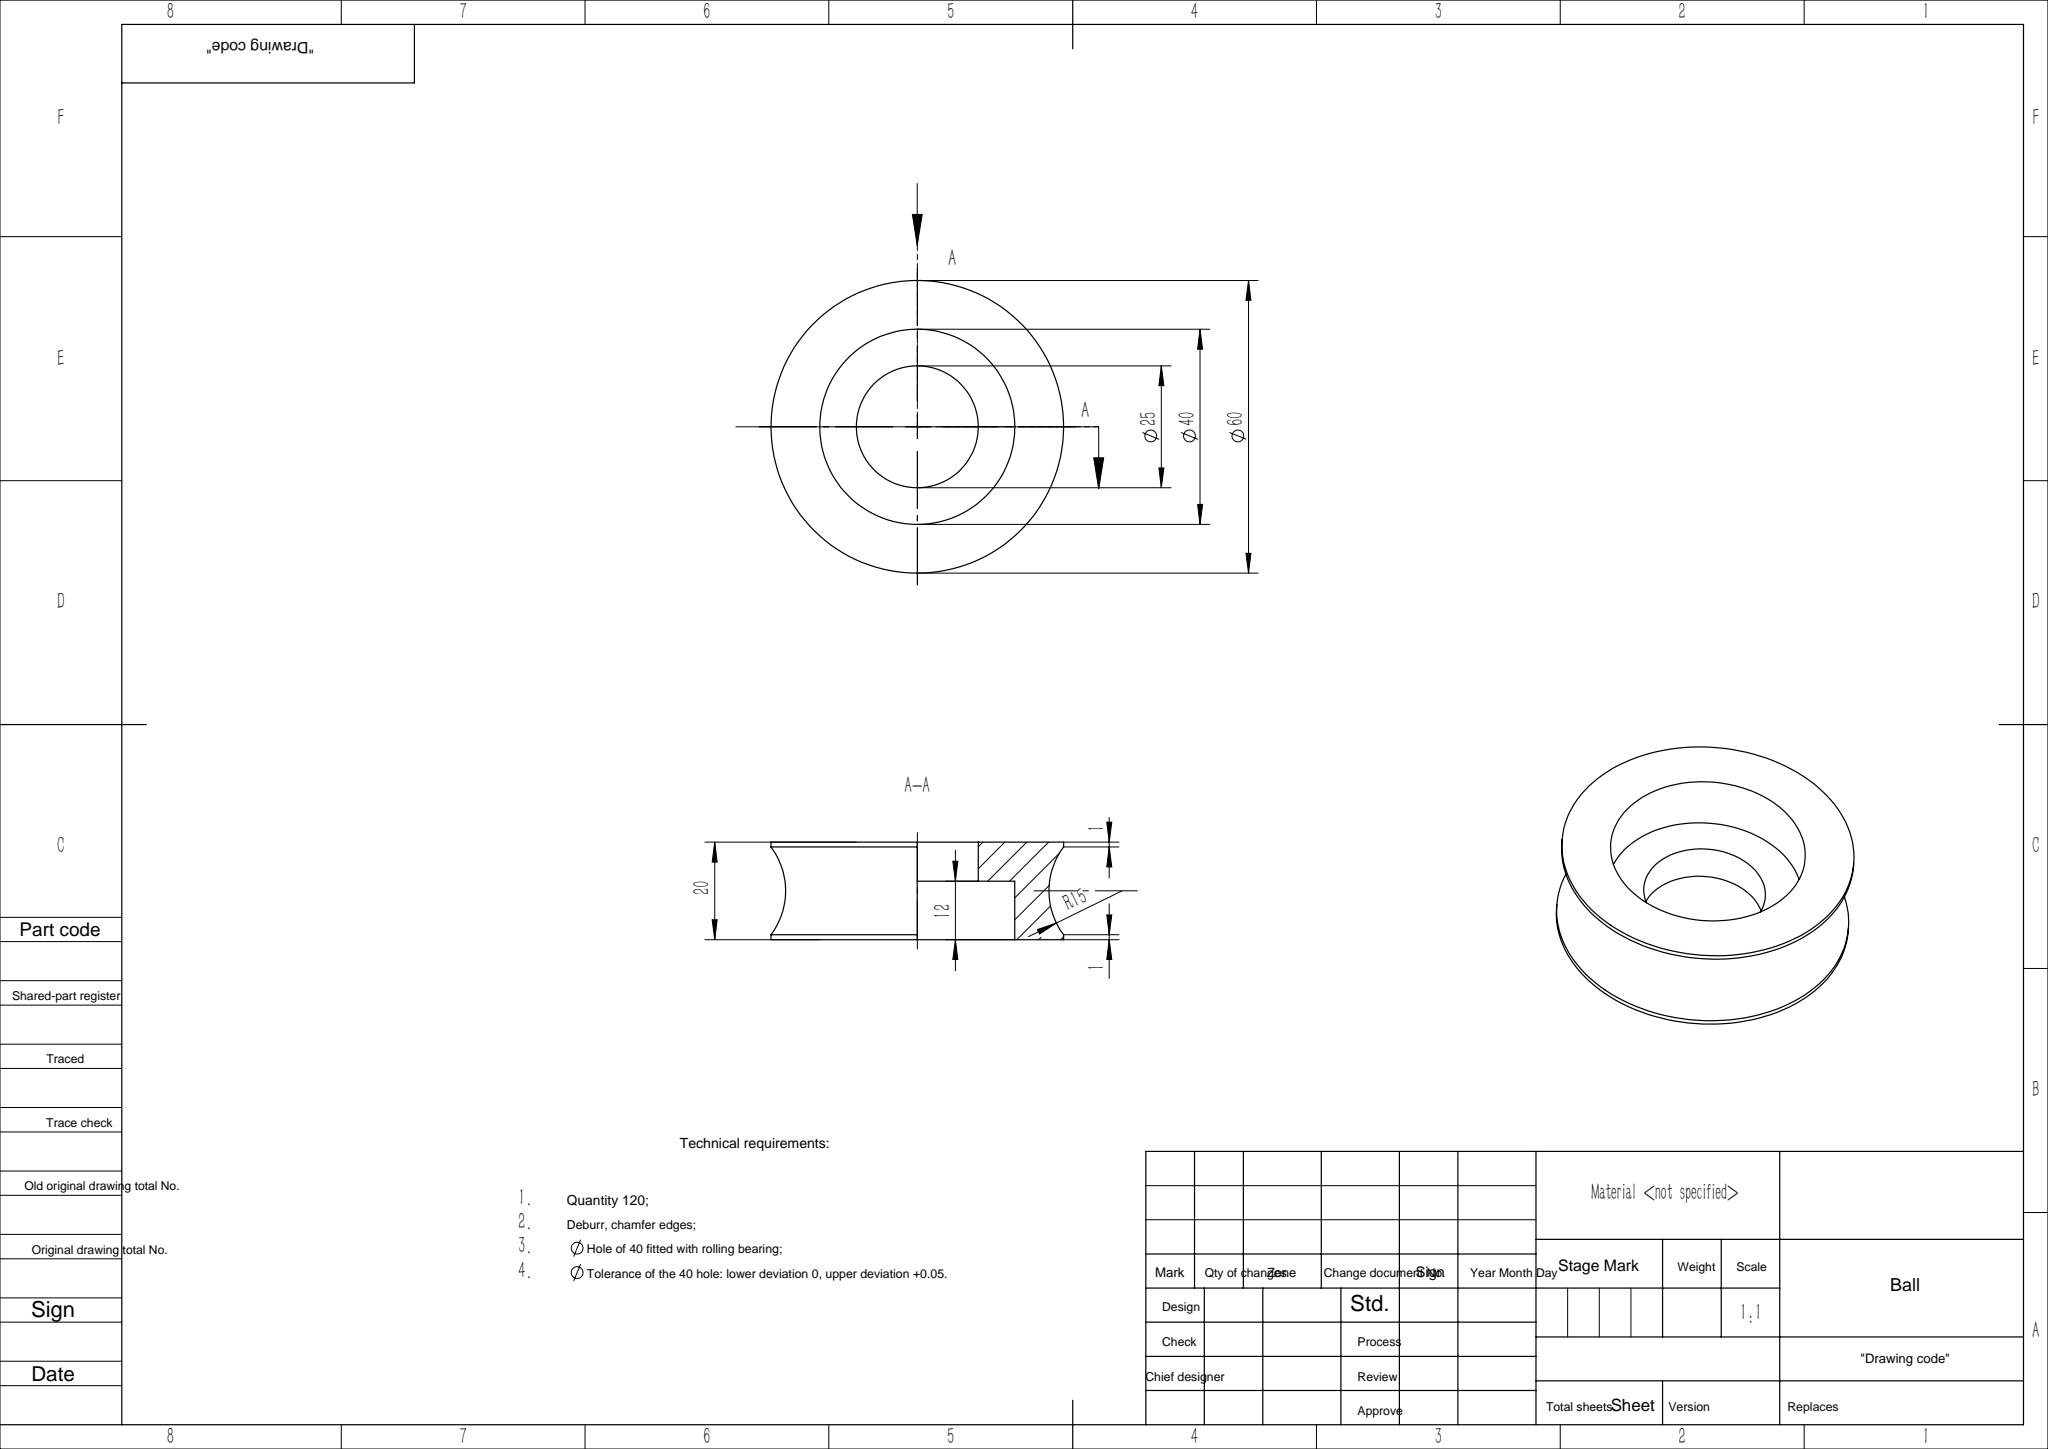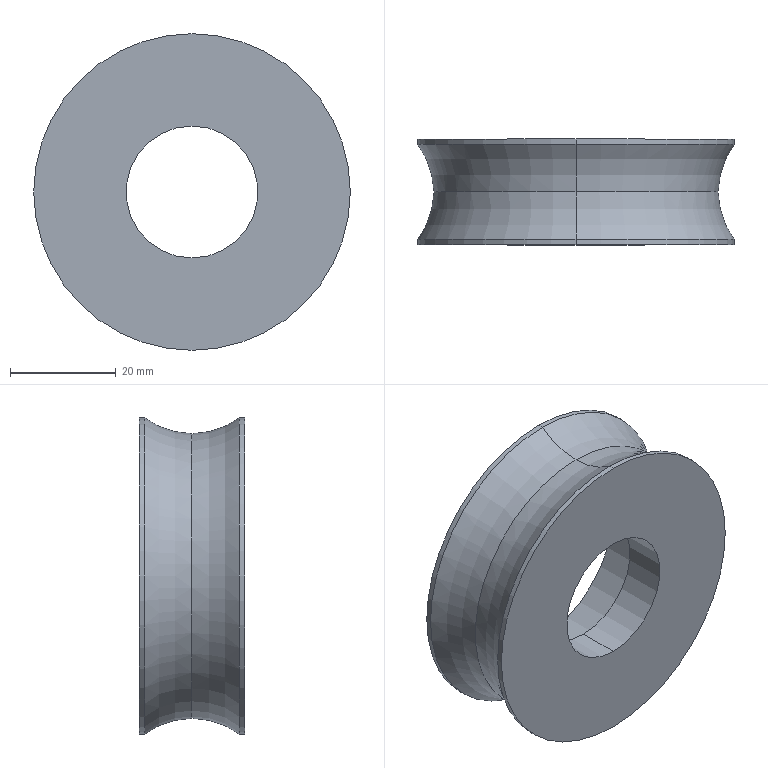Part | SolidWorks | features ICE 2, Extrusion 1, RevCut 1 | 1 solid | 15 faces | box 60 x 20 x 60 mm | volume 30888 mm3 | cylinder 8 | torus 4 | plane 3 | commonest cylinder face diameters 60 x4 25 x2 40 x2
STEP:
#1=CARTESIAN_POINT('',(0.,1.,-30.));
#2=VERTEX_POINT('',#1);
#3=CARTESIAN_POINT('',(0.,10.,-27.));
#4=VERTEX_POINT('',#3);
#5=CARTESIAN_POINT('',(0.,10.,-42.));
#6=DIRECTION('',(-1.,0.,0.));
#7=DIRECTION('',(0.,0.,1.));
#8=AXIS2_PLACEMENT_3D('',#5,#6,#7);
#9=CIRCLE('',#8,15.);
#10=EDGE_CURVE('',#2,#4,#9,.T.);
#11=ORIENTED_EDGE('',*,*,#10,.T.);
#12=CARTESIAN_POINT('',(0.,10.,27.));
#13=VERTEX_POINT('',#12);
#14=CARTESIAN_POINT('',(0.,10.,0.));
#15=DIRECTION('',(0.,-1.,0.));
#16=DIRECTION('',(0.,0.,-1.));
#17=AXIS2_PLACEMENT_3D('',#14,#15,#16);
#18=CIRCLE('',#17,27.);
#19=EDGE_CURVE('',#4,#13,#18,.T.);
#20=ORIENTED_EDGE('',*,*,#19,.T.);
#21=CARTESIAN_POINT('',(0.,1.,30.));
#22=VERTEX_POINT('',#21);
#23=CARTESIAN_POINT('',(0.,10.,42.));
#24=DIRECTION('',(1.,0.,0.));
#25=DIRECTION('',(0.,0.,-1.));
#26=AXIS2_PLACEMENT_3D('',#23,#24,#25);
#27=CIRCLE('',#26,15.);
#28=EDGE_CURVE('',#22,#13,#27,.T.);
#29=ORIENTED_EDGE('',*,*,#28,.F.);
#30=CARTESIAN_POINT('',(0.,1.,0.));
#31=DIRECTION('',(0.,-1.,0.));
#32=DIRECTION('',(0.,0.,1.));
#33=AXIS2_PLACEMENT_3D('',#30,#31,#32);
#34=CIRCLE('',#33,30.);
#35=EDGE_CURVE('',#2,#22,#34,.T.);
#36=ORIENTED_EDGE('',*,*,#35,.F.);
#37=EDGE_LOOP('',(#11,#20,#29,#36));
#38=FACE_OUTER_BOUND('',#37,.T.);
#39=CARTESIAN_POINT('',(0.,10.,0.));
#40=DIRECTION('',(0.,-1.,0.));
#41=DIRECTION('',(0.,0.,-1.));
#42=AXIS2_PLACEMENT_3D('',#39,#40,#41);
#43=TOROIDAL_SURFACE('',#42,42.,15.);
#44=ADVANCED_FACE('',(#38),#43,.F.);
#45=ORIENTED_EDGE('',*,*,#28,.T.);
#46=CARTESIAN_POINT('',(0.,10.,0.));
#47=DIRECTION('',(0.,-1.,0.));
#48=DIRECTION('',(0.,0.,-1.));
#49=AXIS2_PLACEMENT_3D('',#46,#47,#48);
#50=CIRCLE('',#49,27.);
#51=EDGE_CURVE('',#13,#4,#50,.T.);
#52=ORIENTED_EDGE('',*,*,#51,.T.);
#53=ORIENTED_EDGE('',*,*,#10,.F.);
#54=CARTESIAN_POINT('',(0.,1.,0.));
#55=DIRECTION('',(0.,-1.,0.));
#56=DIRECTION('',(0.,0.,1.));
#57=AXIS2_PLACEMENT_3D('',#54,#55,#56);
#58=CIRCLE('',#57,30.);
#59=EDGE_CURVE('',#22,#2,#58,.T.);
#60=ORIENTED_EDGE('',*,*,#59,.F.);
#61=EDGE_LOOP('',(#45,#52,#53,#60));
#62=FACE_OUTER_BOUND('',#61,.T.);
#63=CARTESIAN_POINT('',(0.,10.,0.));
#64=DIRECTION('',(0.,-1.,0.));
#65=DIRECTION('',(0.,0.,-1.));
#66=AXIS2_PLACEMENT_3D('',#63,#64,#65);
#67=TOROIDAL_SURFACE('',#66,42.,15.);
#68=ADVANCED_FACE('',(#62),#67,.F.);
#69=ORIENTED_EDGE('',*,*,#51,.F.);
#70=CARTESIAN_POINT('',(0.,19.,30.));
#71=VERTEX_POINT('',#70);
#72=CARTESIAN_POINT('',(0.,10.,42.));
#73=DIRECTION('',(1.,0.,0.));
#74=DIRECTION('',(0.,0.,-1.));
#75=AXIS2_PLACEMENT_3D('',#72,#73,#74);
#76=CIRCLE('',#75,15.);
#77=EDGE_CURVE('',#13,#71,#76,.T.);
#78=ORIENTED_EDGE('',*,*,#77,.T.);
#79=CARTESIAN_POINT('',(0.,19.,-30.));
#80=VERTEX_POINT('',#79);
#81=CARTESIAN_POINT('',(0.,19.,0.));
#82=DIRECTION('',(0.,1.,0.));
#83=DIRECTION('',(0.,0.,-1.));
#84=AXIS2_PLACEMENT_3D('',#81,#82,#83);
#85=CIRCLE('',#84,30.);
#86=EDGE_CURVE('',#80,#71,#85,.T.);
#87=ORIENTED_EDGE('',*,*,#86,.F.);
#88=CARTESIAN_POINT('',(0.,10.,-42.));
#89=DIRECTION('',(-1.,0.,0.));
#90=DIRECTION('',(0.,0.,1.));
#91=AXIS2_PLACEMENT_3D('',#88,#89,#90);
#92=CIRCLE('',#91,15.);
#93=EDGE_CURVE('',#4,#80,#92,.T.);
#94=ORIENTED_EDGE('',*,*,#93,.F.);
#95=EDGE_LOOP('',(#69,#78,#87,#94));
#96=FACE_OUTER_BOUND('',#95,.T.);
#97=CARTESIAN_POINT('',(0.,10.,0.));
#98=DIRECTION('',(0.,-1.,0.));
#99=DIRECTION('',(0.,0.,-1.));
#100=AXIS2_PLACEMENT_3D('',#97,#98,#99);
#101=TOROIDAL_SURFACE('',#100,42.,15.);
#102=ADVANCED_FACE('',(#96),#101,.F.);
#103=CARTESIAN_POINT('',(0.,0.,-12.5));
#104=VERTEX_POINT('',#103);
#105=CARTESIAN_POINT('',(0.,0.,12.5));
#106=VERTEX_POINT('',#105);
#107=CARTESIAN_POINT('',(0.,0.,0.));
#108=DIRECTION('',(0.,1.,0.));
#109=DIRECTION('',(0.,0.,1.));
#110=AXIS2_PLACEMENT_3D('',#107,#108,#109);
#111=CIRCLE('',#110,12.5);
#112=EDGE_CURVE('',#104,#106,#111,.T.);
#113=ORIENTED_EDGE('',*,*,#112,.F.);
#114=CARTESIAN_POINT('',(0.,8.,-12.5));
#115=VERTEX_POINT('',#114);
#116=CARTESIAN_POINT('',(0.,0.,-12.5));
#117=DIRECTION('',(0.,1.,0.));
#118=VECTOR('',#117,1000.);
#119=LINE('',#116,#118);
#120=EDGE_CURVE('',#104,#115,#119,.T.);
#121=ORIENTED_EDGE('',*,*,#120,.T.);
#122=CARTESIAN_POINT('',(0.,8.,12.5));
#123=VERTEX_POINT('',#122);
#124=CARTESIAN_POINT('',(0.,8.,0.));
#125=DIRECTION('',(0.,1.,0.));
#126=DIRECTION('',(0.,0.,1.));
#127=AXIS2_PLACEMENT_3D('',#124,#125,#126);
#128=CIRCLE('',#127,12.5);
#129=EDGE_CURVE('',#115,#123,#128,.T.);
#130=ORIENTED_EDGE('',*,*,#129,.T.);
#131=CARTESIAN_POINT('',(0.,0.,12.5));
#132=DIRECTION('',(0.,1.,0.));
#133=VECTOR('',#132,1000.);
#134=LINE('',#131,#133);
#135=EDGE_CURVE('',#106,#123,#134,.T.);
#136=ORIENTED_EDGE('',*,*,#135,.F.);
#137=EDGE_LOOP('',(#113,#121,#130,#136));
#138=FACE_OUTER_BOUND('',#137,.T.);
#139=CARTESIAN_POINT('',(0.,0.,0.));
#140=DIRECTION('',(0.,1.,0.));
#141=DIRECTION('',(0.,0.,1.));
#142=AXIS2_PLACEMENT_3D('',#139,#140,#141);
#143=CYLINDRICAL_SURFACE('',#142,12.5);
#144=ADVANCED_FACE('',(#138),#143,.F.);
#145=CARTESIAN_POINT('',(0.,8.,-20.));
#146=VERTEX_POINT('',#145);
#147=CARTESIAN_POINT('',(0.,8.,20.));
#148=VERTEX_POINT('',#147);
#149=CARTESIAN_POINT('',(0.,8.,0.));
#150=DIRECTION('',(0.,1.,0.));
#151=DIRECTION('',(0.,0.,1.));
#152=AXIS2_PLACEMENT_3D('',#149,#150,#151);
#153=CIRCLE('',#152,20.);
#154=EDGE_CURVE('',#146,#148,#153,.T.);
#155=ORIENTED_EDGE('',*,*,#154,.F.);
#156=CARTESIAN_POINT('',(0.,20.,-20.));
#157=VERTEX_POINT('',#156);
#158=CARTESIAN_POINT('',(0.,8.,-20.));
#159=DIRECTION('',(0.,1.,0.));
#160=VECTOR('',#159,1000.);
#161=LINE('',#158,#160);
#162=EDGE_CURVE('',#146,#157,#161,.T.);
#163=ORIENTED_EDGE('',*,*,#162,.T.);
#164=CARTESIAN_POINT('',(0.,20.,20.));
#165=VERTEX_POINT('',#164);
#166=CARTESIAN_POINT('',(0.,20.,0.));
#167=DIRECTION('',(0.,1.,0.));
#168=DIRECTION('',(0.,0.,1.));
#169=AXIS2_PLACEMENT_3D('',#166,#167,#168);
#170=CIRCLE('',#169,20.);
#171=EDGE_CURVE('',#157,#165,#170,.T.);
#172=ORIENTED_EDGE('',*,*,#171,.T.);
#173=CARTESIAN_POINT('',(0.,8.,20.));
#174=DIRECTION('',(0.,1.,0.));
#175=VECTOR('',#174,1000.);
#176=LINE('',#173,#175);
#177=EDGE_CURVE('',#148,#165,#176,.T.);
#178=ORIENTED_EDGE('',*,*,#177,.F.);
#179=EDGE_LOOP('',(#155,#163,#172,#178));
#180=FACE_OUTER_BOUND('',#179,.T.);
#181=CARTESIAN_POINT('',(0.,8.,0.));
#182=DIRECTION('',(0.,1.,0.));
#183=DIRECTION('',(0.,0.,1.));
#184=AXIS2_PLACEMENT_3D('',#181,#182,#183);
#185=CYLINDRICAL_SURFACE('',#184,20.);
#186=ADVANCED_FACE('',(#180),#185,.F.);
#187=CARTESIAN_POINT('',(0.,20.,30.));
#188=VERTEX_POINT('',#187);
#189=CARTESIAN_POINT('',(0.,20.,-30.));
#190=VERTEX_POINT('',#189);
#191=CARTESIAN_POINT('',(0.,20.,0.));
#192=DIRECTION('',(0.,1.,0.));
#193=DIRECTION('',(0.,0.,1.));
#194=AXIS2_PLACEMENT_3D('',#191,#192,#193);
#195=CIRCLE('',#194,30.);
#196=EDGE_CURVE('',#188,#190,#195,.T.);
#197=ORIENTED_EDGE('',*,*,#196,.F.);
#198=CARTESIAN_POINT('',(0.,20.,30.));
#199=DIRECTION('',(0.,-1.,0.));
#200=VECTOR('',#199,1000.);
#201=LINE('',#198,#200);
#202=EDGE_CURVE('',#188,#71,#201,.T.);
#203=ORIENTED_EDGE('',*,*,#202,.T.);
#204=CARTESIAN_POINT('',(0.,19.,0.));
#205=DIRECTION('',(0.,1.,0.));
#206=DIRECTION('',(0.,0.,-1.));
#207=AXIS2_PLACEMENT_3D('',#204,#205,#206);
#208=CIRCLE('',#207,30.);
#209=EDGE_CURVE('',#71,#80,#208,.T.);
#210=ORIENTED_EDGE('',*,*,#209,.T.);
#211=CARTESIAN_POINT('',(0.,20.,-30.));
#212=DIRECTION('',(0.,-1.,0.));
#213=VECTOR('',#212,1000.);
#214=LINE('',#211,#213);
#215=EDGE_CURVE('',#190,#80,#214,.T.);
#216=ORIENTED_EDGE('',*,*,#215,.F.);
#217=EDGE_LOOP('',(#197,#203,#210,#216));
#218=FACE_OUTER_BOUND('',#217,.T.);
#219=CARTESIAN_POINT('',(0.,20.,0.));
#220=DIRECTION('',(0.,-1.,0.));
#221=DIRECTION('',(0.,0.,-1.));
#222=AXIS2_PLACEMENT_3D('',#219,#220,#221);
#223=CYLINDRICAL_SURFACE('',#222,30.);
#224=ADVANCED_FACE('',(#218),#223,.T.);
#225=ORIENTED_EDGE('',*,*,#35,.T.);
#226=CARTESIAN_POINT('',(0.,0.,30.));
#227=VERTEX_POINT('',#226);
#228=CARTESIAN_POINT('',(0.,20.,30.));
#229=DIRECTION('',(0.,-1.,0.));
#230=VECTOR('',#229,1000.);
#231=LINE('',#228,#230);
#232=EDGE_CURVE('',#22,#227,#231,.T.);
#233=ORIENTED_EDGE('',*,*,#232,.T.);
#234=CARTESIAN_POINT('',(0.,0.,-30.));
#235=VERTEX_POINT('',#234);
#236=CARTESIAN_POINT('',(0.,0.,0.));
#237=DIRECTION('',(0.,1.,0.));
#238=DIRECTION('',(0.,0.,1.));
#239=AXIS2_PLACEMENT_3D('',#236,#237,#238);
#240=CIRCLE('',#239,30.);
#241=EDGE_CURVE('',#227,#235,#240,.T.);
#242=ORIENTED_EDGE('',*,*,#241,.T.);
#243=CARTESIAN_POINT('',(0.,20.,-30.));
#244=DIRECTION('',(0.,-1.,0.));
#245=VECTOR('',#244,1000.);
#246=LINE('',#243,#245);
#247=EDGE_CURVE('',#2,#235,#246,.T.);
#248=ORIENTED_EDGE('',*,*,#247,.F.);
#249=EDGE_LOOP('',(#225,#233,#242,#248));
#250=FACE_OUTER_BOUND('',#249,.T.);
#251=CARTESIAN_POINT('',(0.,20.,0.));
#252=DIRECTION('',(0.,-1.,0.));
#253=DIRECTION('',(0.,0.,-1.));
#254=AXIS2_PLACEMENT_3D('',#251,#252,#253);
#255=CYLINDRICAL_SURFACE('',#254,30.);
#256=ADVANCED_FACE('',(#250),#255,.T.);
#257=ORIENTED_EDGE('',*,*,#232,.F.);
#258=ORIENTED_EDGE('',*,*,#59,.T.);
#259=ORIENTED_EDGE('',*,*,#247,.T.);
#260=CARTESIAN_POINT('',(0.,0.,0.));
#261=DIRECTION('',(0.,1.,0.));
#262=DIRECTION('',(0.,0.,1.));
#263=AXIS2_PLACEMENT_3D('',#260,#261,#262);
#264=CIRCLE('',#263,30.);
#265=EDGE_CURVE('',#235,#227,#264,.T.);
#266=ORIENTED_EDGE('',*,*,#265,.T.);
#267=EDGE_LOOP('',(#257,#258,#259,#266));
#268=FACE_OUTER_BOUND('',#267,.T.);
#269=CARTESIAN_POINT('',(0.,20.,0.));
#270=DIRECTION('',(0.,-1.,0.));
#271=DIRECTION('',(0.,0.,-1.));
#272=AXIS2_PLACEMENT_3D('',#269,#270,#271);
#273=CYLINDRICAL_SURFACE('',#272,30.);
#274=ADVANCED_FACE('',(#268),#273,.T.);
#275=ORIENTED_EDGE('',*,*,#202,.F.);
#276=CARTESIAN_POINT('',(0.,20.,0.));
#277=DIRECTION('',(0.,1.,0.));
#278=DIRECTION('',(0.,0.,1.));
#279=AXIS2_PLACEMENT_3D('',#276,#277,#278);
#280=CIRCLE('',#279,30.);
#281=EDGE_CURVE('',#190,#188,#280,.T.);
#282=ORIENTED_EDGE('',*,*,#281,.F.);
#283=ORIENTED_EDGE('',*,*,#215,.T.);
#284=ORIENTED_EDGE('',*,*,#86,.T.);
#285=EDGE_LOOP('',(#275,#282,#283,#284));
#286=FACE_OUTER_BOUND('',#285,.T.);
#287=CARTESIAN_POINT('',(0.,20.,0.));
#288=DIRECTION('',(0.,-1.,0.));
#289=DIRECTION('',(0.,0.,-1.));
#290=AXIS2_PLACEMENT_3D('',#287,#288,#289);
#291=CYLINDRICAL_SURFACE('',#290,30.);
#292=ADVANCED_FACE('',(#286),#291,.T.);
#293=CARTESIAN_POINT('',(0.,20.,0.));
#294=DIRECTION('',(0.,1.,0.));
#295=DIRECTION('',(0.,0.,1.));
#296=AXIS2_PLACEMENT_3D('',#293,#294,#295);
#297=CIRCLE('',#296,20.);
#298=EDGE_CURVE('',#165,#157,#297,.T.);
#299=ORIENTED_EDGE('',*,*,#298,.F.);
#300=ORIENTED_EDGE('',*,*,#171,.F.);
#301=EDGE_LOOP('',(#299,#300));
#302=FACE_BOUND('',#301,.T.);
#303=ORIENTED_EDGE('',*,*,#281,.T.);
#304=ORIENTED_EDGE('',*,*,#196,.T.);
#305=EDGE_LOOP('',(#303,#304));
#306=FACE_OUTER_BOUND('',#305,.T.);
#307=CARTESIAN_POINT('',(0.,20.,0.));
#308=DIRECTION('',(0.,1.,0.));
#309=DIRECTION('',(0.,0.,1.));
#310=AXIS2_PLACEMENT_3D('',#307,#308,#309);
#311=PLANE('',#310);
#312=ADVANCED_FACE('',(#302,#306),#311,.T.);
#313=CARTESIAN_POINT('',(0.,0.,0.));
#314=DIRECTION('',(0.,1.,0.));
#315=DIRECTION('',(0.,0.,1.));
#316=AXIS2_PLACEMENT_3D('',#313,#314,#315);
#317=CIRCLE('',#316,12.5);
#318=EDGE_CURVE('',#106,#104,#317,.T.);
#319=ORIENTED_EDGE('',*,*,#318,.T.);
#320=ORIENTED_EDGE('',*,*,#112,.T.);
#321=EDGE_LOOP('',(#319,#320));
#322=FACE_BOUND('',#321,.T.);
#323=ORIENTED_EDGE('',*,*,#265,.F.);
#324=ORIENTED_EDGE('',*,*,#241,.F.);
#325=EDGE_LOOP('',(#323,#324));
#326=FACE_OUTER_BOUND('',#325,.T.);
#327=CARTESIAN_POINT('',(0.,0.,0.));
#328=DIRECTION('',(0.,1.,0.));
#329=DIRECTION('',(0.,0.,1.));
#330=AXIS2_PLACEMENT_3D('',#327,#328,#329);
#331=PLANE('',#330);
#332=ADVANCED_FACE('',(#322,#326),#331,.F.);
#333=ORIENTED_EDGE('',*,*,#162,.F.);
#334=CARTESIAN_POINT('',(0.,8.,0.));
#335=DIRECTION('',(0.,1.,0.));
#336=DIRECTION('',(0.,0.,1.));
#337=AXIS2_PLACEMENT_3D('',#334,#335,#336);
#338=CIRCLE('',#337,20.);
#339=EDGE_CURVE('',#148,#146,#338,.T.);
#340=ORIENTED_EDGE('',*,*,#339,.F.);
#341=ORIENTED_EDGE('',*,*,#177,.T.);
#342=ORIENTED_EDGE('',*,*,#298,.T.);
#343=EDGE_LOOP('',(#333,#340,#341,#342));
#344=FACE_OUTER_BOUND('',#343,.T.);
#345=CARTESIAN_POINT('',(0.,8.,0.));
#346=DIRECTION('',(0.,1.,0.));
#347=DIRECTION('',(0.,0.,1.));
#348=AXIS2_PLACEMENT_3D('',#345,#346,#347);
#349=CYLINDRICAL_SURFACE('',#348,20.);
#350=ADVANCED_FACE('',(#344),#349,.F.);
#351=CARTESIAN_POINT('',(0.,8.,0.));
#352=DIRECTION('',(0.,1.,0.));
#353=DIRECTION('',(0.,0.,1.));
#354=AXIS2_PLACEMENT_3D('',#351,#352,#353);
#355=CIRCLE('',#354,12.5);
#356=EDGE_CURVE('',#123,#115,#355,.T.);
#357=ORIENTED_EDGE('',*,*,#356,.F.);
#358=ORIENTED_EDGE('',*,*,#129,.F.);
#359=EDGE_LOOP('',(#357,#358));
#360=FACE_BOUND('',#359,.T.);
#361=ORIENTED_EDGE('',*,*,#339,.T.);
#362=ORIENTED_EDGE('',*,*,#154,.T.);
#363=EDGE_LOOP('',(#361,#362));
#364=FACE_OUTER_BOUND('',#363,.T.);
#365=CARTESIAN_POINT('',(0.,8.,0.));
#366=DIRECTION('',(0.,1.,0.));
#367=DIRECTION('',(0.,0.,1.));
#368=AXIS2_PLACEMENT_3D('',#365,#366,#367);
#369=PLANE('',#368);
#370=ADVANCED_FACE('',(#360,#364),#369,.T.);
#371=ORIENTED_EDGE('',*,*,#120,.F.);
#372=ORIENTED_EDGE('',*,*,#318,.F.);
#373=ORIENTED_EDGE('',*,*,#135,.T.);
#374=ORIENTED_EDGE('',*,*,#356,.T.);
#375=EDGE_LOOP('',(#371,#372,#373,#374));
#376=FACE_OUTER_BOUND('',#375,.T.);
#377=CARTESIAN_POINT('',(0.,0.,0.));
#378=DIRECTION('',(0.,1.,0.));
#379=DIRECTION('',(0.,0.,1.));
#380=AXIS2_PLACEMENT_3D('',#377,#378,#379);
#381=CYLINDRICAL_SURFACE('',#380,12.5);
#382=ADVANCED_FACE('',(#376),#381,.F.);
#383=ORIENTED_EDGE('',*,*,#19,.F.);
#384=ORIENTED_EDGE('',*,*,#93,.T.);
#385=ORIENTED_EDGE('',*,*,#209,.F.);
#386=ORIENTED_EDGE('',*,*,#77,.F.);
#387=EDGE_LOOP('',(#383,#384,#385,#386));
#388=FACE_OUTER_BOUND('',#387,.T.);
#389=CARTESIAN_POINT('',(0.,10.,0.));
#390=DIRECTION('',(0.,-1.,0.));
#391=DIRECTION('',(0.,0.,-1.));
#392=AXIS2_PLACEMENT_3D('',#389,#390,#391);
#393=TOROIDAL_SURFACE('',#392,42.,15.);
#394=ADVANCED_FACE('',(#388),#393,.F.);
#395=CLOSED_SHELL('',(#44,#68,#102,#144,#186,#224,#256,#274,#292,#312,#332,#350,#370,#382,#394));
#396=MANIFOLD_SOLID_BREP('',#395);
#397=CARTESIAN_POINT('',(0.,0.,0.));
#398=DIRECTION('',(0.,0.,1.));
#399=DIRECTION('',(1.,0.,0.));
#400=AXIS2_PLACEMENT_3D('',#397,#398,#399);
#401=(LENGTH_UNIT()NAMED_UNIT(*)SI_UNIT(.MILLI.,.METRE.));
#402=UNCERTAINTY_MEASURE_WITH_UNIT(LENGTH_MEASURE(0.00001),#401,'','');
#403=(NAMED_UNIT(*)PLANE_ANGLE_UNIT()SI_UNIT($,.RADIAN.));
#404=(NAMED_UNIT(*)SI_UNIT($,.STERADIAN.)SOLID_ANGLE_UNIT());
#405=(GEOMETRIC_REPRESENTATION_CONTEXT(3)GLOBAL_UNCERTAINTY_ASSIGNED_CONTEXT((#402))GLOBAL_UNIT_ASSIGNED_CONTEXT((#401,#403,#404))REPRESENTATION_CONTEXT('',''));
#406=ADVANCED_BREP_SHAPE_REPRESENTATION('',(#396,#400),#405);